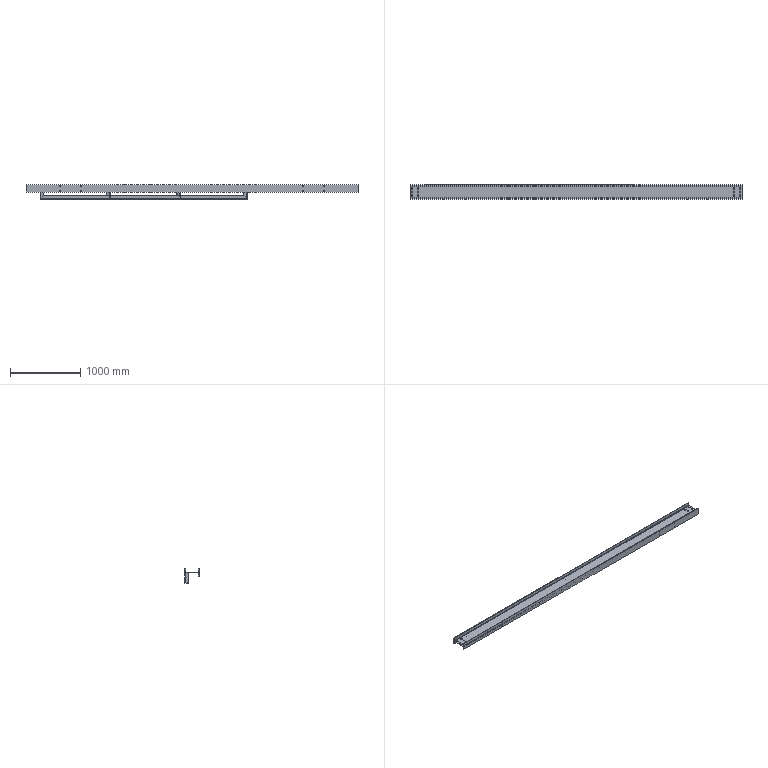Part | STEP file | Landing main beam 4 body_Default<As Machined> | 6 solids | 131 faces | box 4730 x 200 x 200 mm | volume 13878197 mm3 | plane 72 | cylinder 59 | commonest cylinder face diameters 19 x24 15 x16 2.66 x10 11 x5 16 x4